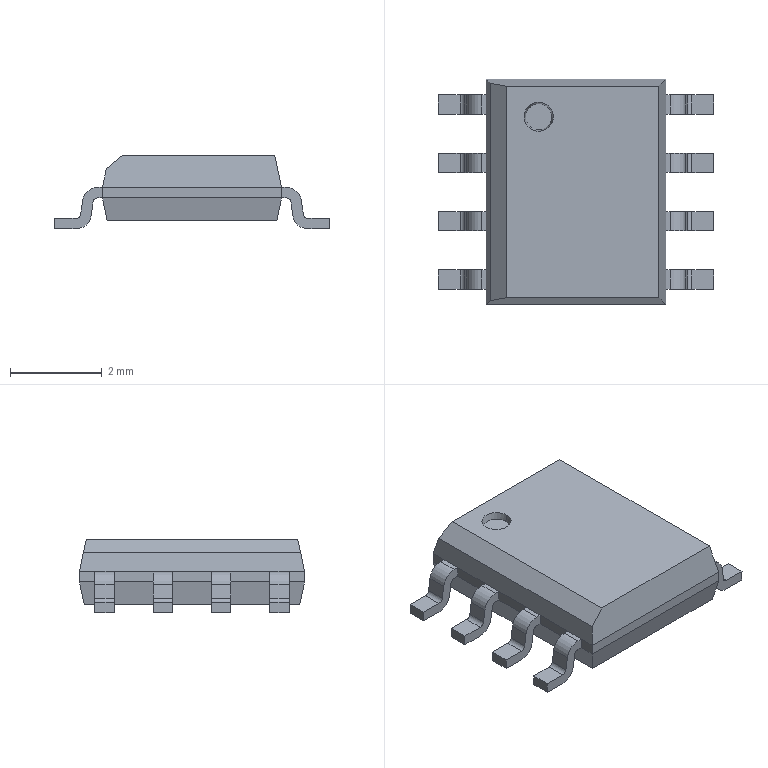Part | STEP file | RJ-USIO-V1_2-220411_116 | 1 solid | 130 faces | box 5.99 x 4.9 x 1.6 mm | volume 26.711 mm3 | plane 96 | cylinder 32 | cone 2 | commonest cylinder face diameters 0.2 x16 0.66 x16